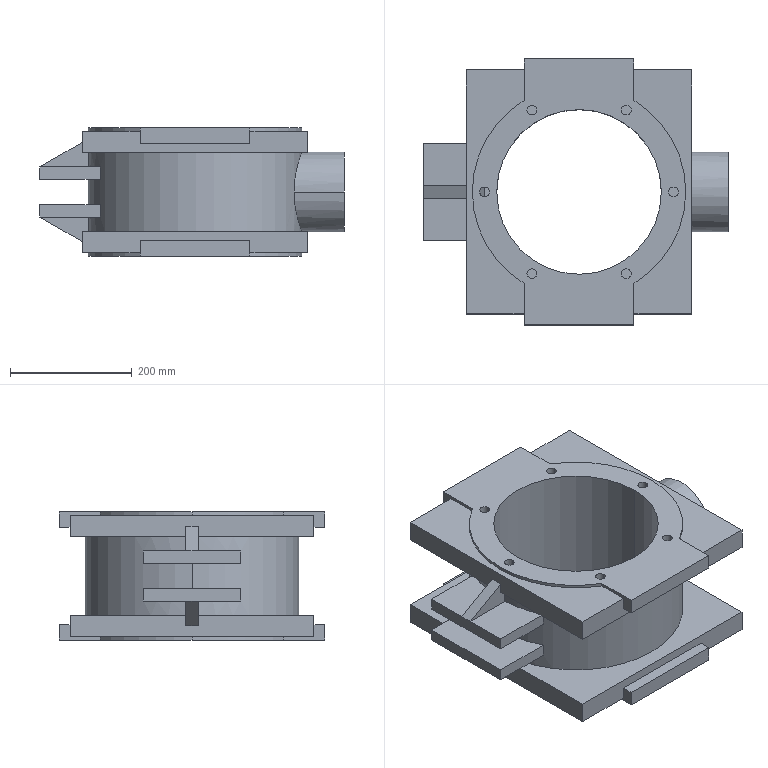Part | NX | features BREP 1 | 1 solid | 108 faces | box 500 x 436 x 210 mm | volume 13297149 mm3 | plane 69 | cylinder 39 | commonest cylinder face diameters 16 x24 350 x9 91 x2 131 x2 270 x2